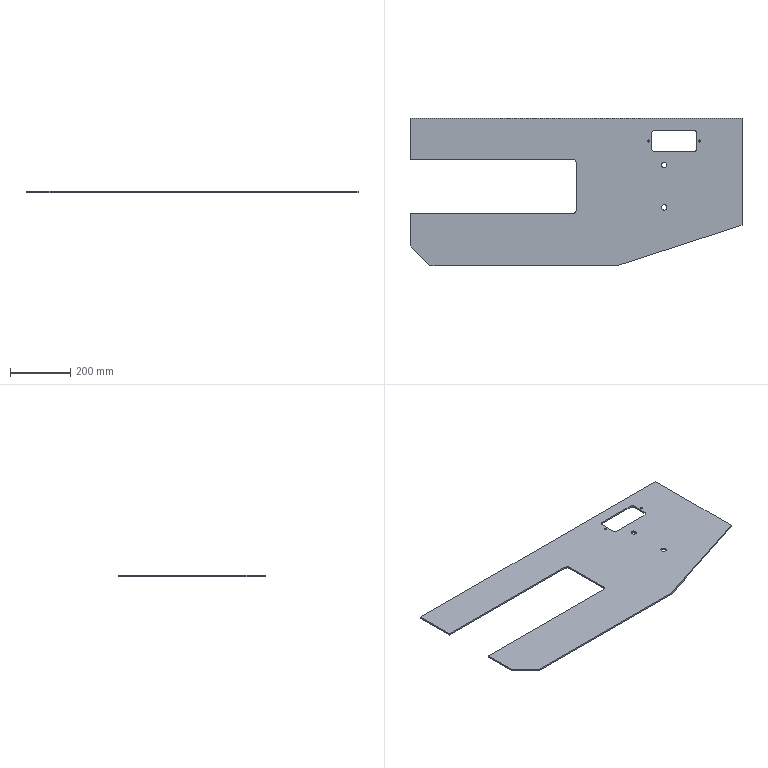Part | SolidWorks | features HoleWzd 2, FlatPattern 1, SMBaseFlange 1, SheetMetal 1 | 1 solid | 30 faces | box 1100 x 490 x 5 mm | volume 1994925 mm3 | plane 16 | cylinder 14 | commonest cylinder face diameters 20 x6 6.8 x4 17.5 x4
STEP:
#1=CARTESIAN_POINT('',(786.6,414.,-5.));
#2=VERTEX_POINT('',#1);
#3=CARTESIAN_POINT('',(793.4,414.,-5.));
#4=VERTEX_POINT('',#3);
#5=CARTESIAN_POINT('',(790.,414.,-5.));
#6=DIRECTION('',(0.,0.,1.));
#7=DIRECTION('',(1.,0.,0.));
#8=AXIS2_PLACEMENT_3D('',#5,#6,#7);
#9=CIRCLE('',#8,3.4);
#10=EDGE_CURVE('',#2,#4,#9,.T.);
#11=ORIENTED_EDGE('',*,*,#10,.F.);
#12=CARTESIAN_POINT('',(786.6,414.,0.));
#13=VERTEX_POINT('',#12);
#14=CARTESIAN_POINT('',(786.6,414.,0.));
#15=DIRECTION('',(0.,0.,1.));
#16=VECTOR('',#15,1000.);
#17=LINE('',#14,#16);
#18=EDGE_CURVE('',#2,#13,#17,.T.);
#19=ORIENTED_EDGE('',*,*,#18,.T.);
#20=CARTESIAN_POINT('',(793.4,414.,0.));
#21=VERTEX_POINT('',#20);
#22=CARTESIAN_POINT('',(790.,414.,0.));
#23=DIRECTION('',(0.,0.,1.));
#24=DIRECTION('',(1.,0.,0.));
#25=AXIS2_PLACEMENT_3D('',#22,#23,#24);
#26=CIRCLE('',#25,3.4);
#27=EDGE_CURVE('',#13,#21,#26,.T.);
#28=ORIENTED_EDGE('',*,*,#27,.T.);
#29=CARTESIAN_POINT('',(793.4,414.,0.));
#30=DIRECTION('',(0.,0.,1.));
#31=VECTOR('',#30,1000.);
#32=LINE('',#29,#31);
#33=EDGE_CURVE('',#4,#21,#32,.T.);
#34=ORIENTED_EDGE('',*,*,#33,.F.);
#35=EDGE_LOOP('',(#11,#19,#28,#34));
#36=FACE_OUTER_BOUND('',#35,.T.);
#37=CARTESIAN_POINT('',(790.,414.,0.));
#38=DIRECTION('',(0.,0.,1.));
#39=DIRECTION('',(1.,0.,0.));
#40=AXIS2_PLACEMENT_3D('',#37,#38,#39);
#41=CYLINDRICAL_SURFACE('',#40,3.4);
#42=ADVANCED_FACE('',(#36),#41,.F.);
#43=CARTESIAN_POINT('',(956.6,414.,-5.));
#44=VERTEX_POINT('',#43);
#45=CARTESIAN_POINT('',(963.4,414.,-5.));
#46=VERTEX_POINT('',#45);
#47=CARTESIAN_POINT('',(960.,414.,-5.));
#48=DIRECTION('',(0.,0.,1.));
#49=DIRECTION('',(1.,0.,0.));
#50=AXIS2_PLACEMENT_3D('',#47,#48,#49);
#51=CIRCLE('',#50,3.4);
#52=EDGE_CURVE('',#44,#46,#51,.T.);
#53=ORIENTED_EDGE('',*,*,#52,.F.);
#54=CARTESIAN_POINT('',(956.6,414.,0.));
#55=VERTEX_POINT('',#54);
#56=CARTESIAN_POINT('',(956.6,414.,0.));
#57=DIRECTION('',(0.,0.,1.));
#58=VECTOR('',#57,1000.);
#59=LINE('',#56,#58);
#60=EDGE_CURVE('',#44,#55,#59,.T.);
#61=ORIENTED_EDGE('',*,*,#60,.T.);
#62=CARTESIAN_POINT('',(963.4,414.,0.));
#63=VERTEX_POINT('',#62);
#64=CARTESIAN_POINT('',(960.,414.,0.));
#65=DIRECTION('',(0.,0.,1.));
#66=DIRECTION('',(1.,0.,0.));
#67=AXIS2_PLACEMENT_3D('',#64,#65,#66);
#68=CIRCLE('',#67,3.4);
#69=EDGE_CURVE('',#55,#63,#68,.T.);
#70=ORIENTED_EDGE('',*,*,#69,.T.);
#71=CARTESIAN_POINT('',(963.4,414.,0.));
#72=DIRECTION('',(0.,0.,1.));
#73=VECTOR('',#72,1000.);
#74=LINE('',#71,#73);
#75=EDGE_CURVE('',#46,#63,#74,.T.);
#76=ORIENTED_EDGE('',*,*,#75,.F.);
#77=EDGE_LOOP('',(#53,#61,#70,#76));
#78=FACE_OUTER_BOUND('',#77,.T.);
#79=CARTESIAN_POINT('',(960.,414.,0.));
#80=DIRECTION('',(0.,0.,1.));
#81=DIRECTION('',(1.,0.,0.));
#82=AXIS2_PLACEMENT_3D('',#79,#80,#81);
#83=CYLINDRICAL_SURFACE('',#82,3.4);
#84=ADVANCED_FACE('',(#78),#83,.F.);
#85=CARTESIAN_POINT('',(833.25,334.,-5.));
#86=VERTEX_POINT('',#85);
#87=CARTESIAN_POINT('',(850.75,334.,-5.));
#88=VERTEX_POINT('',#87);
#89=CARTESIAN_POINT('',(842.,334.,-5.));
#90=DIRECTION('',(0.,0.,1.));
#91=DIRECTION('',(1.,0.,0.));
#92=AXIS2_PLACEMENT_3D('',#89,#90,#91);
#93=CIRCLE('',#92,8.75);
#94=EDGE_CURVE('',#86,#88,#93,.T.);
#95=ORIENTED_EDGE('',*,*,#94,.F.);
#96=CARTESIAN_POINT('',(833.25,334.,0.));
#97=VERTEX_POINT('',#96);
#98=CARTESIAN_POINT('',(833.25,334.,0.));
#99=DIRECTION('',(0.,0.,1.));
#100=VECTOR('',#99,1000.);
#101=LINE('',#98,#100);
#102=EDGE_CURVE('',#86,#97,#101,.T.);
#103=ORIENTED_EDGE('',*,*,#102,.T.);
#104=CARTESIAN_POINT('',(850.75,334.,0.));
#105=VERTEX_POINT('',#104);
#106=CARTESIAN_POINT('',(842.,334.,0.));
#107=DIRECTION('',(0.,0.,1.));
#108=DIRECTION('',(1.,0.,0.));
#109=AXIS2_PLACEMENT_3D('',#106,#107,#108);
#110=CIRCLE('',#109,8.75);
#111=EDGE_CURVE('',#97,#105,#110,.T.);
#112=ORIENTED_EDGE('',*,*,#111,.T.);
#113=CARTESIAN_POINT('',(850.75,334.,0.));
#114=DIRECTION('',(0.,0.,1.));
#115=VECTOR('',#114,1000.);
#116=LINE('',#113,#115);
#117=EDGE_CURVE('',#88,#105,#116,.T.);
#118=ORIENTED_EDGE('',*,*,#117,.F.);
#119=EDGE_LOOP('',(#95,#103,#112,#118));
#120=FACE_OUTER_BOUND('',#119,.T.);
#121=CARTESIAN_POINT('',(842.,334.,0.));
#122=DIRECTION('',(0.,0.,1.));
#123=DIRECTION('',(1.,0.,0.));
#124=AXIS2_PLACEMENT_3D('',#121,#122,#123);
#125=CYLINDRICAL_SURFACE('',#124,8.75);
#126=ADVANCED_FACE('',(#120),#125,.F.);
#127=CARTESIAN_POINT('',(833.25,194.,-5.));
#128=VERTEX_POINT('',#127);
#129=CARTESIAN_POINT('',(850.75,194.,-5.));
#130=VERTEX_POINT('',#129);
#131=CARTESIAN_POINT('',(842.,194.,-5.));
#132=DIRECTION('',(0.,0.,1.));
#133=DIRECTION('',(1.,0.,0.));
#134=AXIS2_PLACEMENT_3D('',#131,#132,#133);
#135=CIRCLE('',#134,8.75);
#136=EDGE_CURVE('',#128,#130,#135,.T.);
#137=ORIENTED_EDGE('',*,*,#136,.F.);
#138=CARTESIAN_POINT('',(833.25,194.,0.));
#139=VERTEX_POINT('',#138);
#140=CARTESIAN_POINT('',(833.25,194.,0.));
#141=DIRECTION('',(0.,0.,1.));
#142=VECTOR('',#141,1000.);
#143=LINE('',#140,#142);
#144=EDGE_CURVE('',#128,#139,#143,.T.);
#145=ORIENTED_EDGE('',*,*,#144,.T.);
#146=CARTESIAN_POINT('',(850.75,194.,0.));
#147=VERTEX_POINT('',#146);
#148=CARTESIAN_POINT('',(842.,194.,0.));
#149=DIRECTION('',(0.,0.,1.));
#150=DIRECTION('',(1.,0.,0.));
#151=AXIS2_PLACEMENT_3D('',#148,#149,#150);
#152=CIRCLE('',#151,8.75);
#153=EDGE_CURVE('',#139,#147,#152,.T.);
#154=ORIENTED_EDGE('',*,*,#153,.T.);
#155=CARTESIAN_POINT('',(850.75,194.,0.));
#156=DIRECTION('',(0.,0.,1.));
#157=VECTOR('',#156,1000.);
#158=LINE('',#155,#157);
#159=EDGE_CURVE('',#130,#147,#158,.T.);
#160=ORIENTED_EDGE('',*,*,#159,.F.);
#161=EDGE_LOOP('',(#137,#145,#154,#160));
#162=FACE_OUTER_BOUND('',#161,.T.);
#163=CARTESIAN_POINT('',(842.,194.,0.));
#164=DIRECTION('',(0.,0.,1.));
#165=DIRECTION('',(1.,0.,0.));
#166=AXIS2_PLACEMENT_3D('',#163,#164,#165);
#167=CYLINDRICAL_SURFACE('',#166,8.75);
#168=ADVANCED_FACE('',(#162),#167,.F.);
#169=CARTESIAN_POINT('',(0.,490.,0.));
#170=VERTEX_POINT('',#169);
#171=CARTESIAN_POINT('',(0.,354.,0.));
#172=VERTEX_POINT('',#171);
#173=CARTESIAN_POINT('',(0.,354.,0.));
#174=DIRECTION('',(0.,-1.,0.));
#175=VECTOR('',#174,1000.);
#176=LINE('',#173,#175);
#177=EDGE_CURVE('',#170,#172,#176,.T.);
#178=ORIENTED_EDGE('',*,*,#177,.F.);
#179=CARTESIAN_POINT('',(0.,490.,-5.));
#180=VERTEX_POINT('',#179);
#181=CARTESIAN_POINT('',(0.,490.,-5.));
#182=DIRECTION('',(0.,0.,1.));
#183=VECTOR('',#182,1000.);
#184=LINE('',#181,#183);
#185=EDGE_CURVE('',#180,#170,#184,.T.);
#186=ORIENTED_EDGE('',*,*,#185,.F.);
#187=CARTESIAN_POINT('',(0.,354.,-5.));
#188=VERTEX_POINT('',#187);
#189=CARTESIAN_POINT('',(0.,354.,-5.));
#190=DIRECTION('',(0.,-1.,0.));
#191=VECTOR('',#190,1000.);
#192=LINE('',#189,#191);
#193=EDGE_CURVE('',#180,#188,#192,.T.);
#194=ORIENTED_EDGE('',*,*,#193,.T.);
#195=CARTESIAN_POINT('',(0.,354.,-5.));
#196=DIRECTION('',(0.,0.,1.));
#197=VECTOR('',#196,1000.);
#198=LINE('',#195,#197);
#199=EDGE_CURVE('',#188,#172,#198,.T.);
#200=ORIENTED_EDGE('',*,*,#199,.T.);
#201=EDGE_LOOP('',(#178,#186,#194,#200));
#202=FACE_OUTER_BOUND('',#201,.T.);
#203=CARTESIAN_POINT('',(0.,354.,-5.));
#204=DIRECTION('',(-1.,0.,0.));
#205=DIRECTION('',(0.,-1.,0.));
#206=AXIS2_PLACEMENT_3D('',#203,#204,#205);
#207=PLANE('',#206);
#208=ADVANCED_FACE('',(#202),#207,.T.);
#209=CARTESIAN_POINT('',(1100.,490.,0.));
#210=VERTEX_POINT('',#209);
#211=CARTESIAN_POINT('',(0.,490.,0.));
#212=DIRECTION('',(-1.,0.,0.));
#213=VECTOR('',#212,1000.);
#214=LINE('',#211,#213);
#215=EDGE_CURVE('',#210,#170,#214,.T.);
#216=ORIENTED_EDGE('',*,*,#215,.F.);
#217=CARTESIAN_POINT('',(1100.,490.,-5.));
#218=VERTEX_POINT('',#217);
#219=CARTESIAN_POINT('',(1100.,490.,-5.));
#220=DIRECTION('',(0.,0.,1.));
#221=VECTOR('',#220,1000.);
#222=LINE('',#219,#221);
#223=EDGE_CURVE('',#218,#210,#222,.T.);
#224=ORIENTED_EDGE('',*,*,#223,.F.);
#225=CARTESIAN_POINT('',(0.,490.,-5.));
#226=DIRECTION('',(-1.,0.,0.));
#227=VECTOR('',#226,1000.);
#228=LINE('',#225,#227);
#229=EDGE_CURVE('',#218,#180,#228,.T.);
#230=ORIENTED_EDGE('',*,*,#229,.T.);
#231=ORIENTED_EDGE('',*,*,#185,.T.);
#232=EDGE_LOOP('',(#216,#224,#230,#231));
#233=FACE_OUTER_BOUND('',#232,.T.);
#234=CARTESIAN_POINT('',(0.,490.,-5.));
#235=DIRECTION('',(0.,1.,0.));
#236=DIRECTION('',(0.,0.,1.));
#237=AXIS2_PLACEMENT_3D('',#234,#235,#236);
#238=PLANE('',#237);
#239=ADVANCED_FACE('',(#233),#238,.T.);
#240=CARTESIAN_POINT('',(1100.,134.647,0.));
#241=VERTEX_POINT('',#240);
#242=CARTESIAN_POINT('',(1100.,490.,0.));
#243=DIRECTION('',(0.,1.,0.));
#244=VECTOR('',#243,1000.);
#245=LINE('',#242,#244);
#246=EDGE_CURVE('',#241,#210,#245,.T.);
#247=ORIENTED_EDGE('',*,*,#246,.F.);
#248=CARTESIAN_POINT('',(1100.,134.647,-5.));
#249=VERTEX_POINT('',#248);
#250=CARTESIAN_POINT('',(1100.,134.647,-5.));
#251=DIRECTION('',(0.,0.,1.));
#252=VECTOR('',#251,1000.);
#253=LINE('',#250,#252);
#254=EDGE_CURVE('',#249,#241,#253,.T.);
#255=ORIENTED_EDGE('',*,*,#254,.F.);
#256=CARTESIAN_POINT('',(1100.,490.,-5.));
#257=DIRECTION('',(0.,1.,0.));
#258=VECTOR('',#257,1000.);
#259=LINE('',#256,#258);
#260=EDGE_CURVE('',#249,#218,#259,.T.);
#261=ORIENTED_EDGE('',*,*,#260,.T.);
#262=ORIENTED_EDGE('',*,*,#223,.T.);
#263=EDGE_LOOP('',(#247,#255,#261,#262));
#264=FACE_OUTER_BOUND('',#263,.T.);
#265=CARTESIAN_POINT('',(1100.,490.,-5.));
#266=DIRECTION('',(1.,0.,0.));
#267=DIRECTION('',(0.,0.,-1.));
#268=AXIS2_PLACEMENT_3D('',#265,#266,#267);
#269=PLANE('',#268);
#270=ADVANCED_FACE('',(#264),#269,.T.);
#271=CARTESIAN_POINT('',(685.6,0.,0.));
#272=VERTEX_POINT('',#271);
#273=CARTESIAN_POINT('',(1100.,134.647,0.));
#274=DIRECTION('',(0.9511,0.309,0.));
#275=VECTOR('',#274,1000.);
#276=LINE('',#273,#275);
#277=EDGE_CURVE('',#272,#241,#276,.T.);
#278=ORIENTED_EDGE('',*,*,#277,.F.);
#279=CARTESIAN_POINT('',(685.6,0.,-5.));
#280=VERTEX_POINT('',#279);
#281=CARTESIAN_POINT('',(685.6,0.,-5.));
#282=DIRECTION('',(0.,0.,1.));
#283=VECTOR('',#282,1000.);
#284=LINE('',#281,#283);
#285=EDGE_CURVE('',#280,#272,#284,.T.);
#286=ORIENTED_EDGE('',*,*,#285,.F.);
#287=CARTESIAN_POINT('',(1100.,134.647,-5.));
#288=DIRECTION('',(0.9511,0.309,0.));
#289=VECTOR('',#288,1000.);
#290=LINE('',#287,#289);
#291=EDGE_CURVE('',#280,#249,#290,.T.);
#292=ORIENTED_EDGE('',*,*,#291,.T.);
#293=ORIENTED_EDGE('',*,*,#254,.T.);
#294=EDGE_LOOP('',(#278,#286,#292,#293));
#295=FACE_OUTER_BOUND('',#294,.T.);
#296=CARTESIAN_POINT('',(1100.,134.647,-5.));
#297=DIRECTION('',(0.309,-0.9511,0.));
#298=DIRECTION('',(0.9511,0.309,0.));
#299=AXIS2_PLACEMENT_3D('',#296,#297,#298);
#300=PLANE('',#299);
#301=ADVANCED_FACE('',(#295),#300,.T.);
#302=CARTESIAN_POINT('',(66.2,0.,0.));
#303=VERTEX_POINT('',#302);
#304=CARTESIAN_POINT('',(685.6,0.,0.));
#305=DIRECTION('',(1.,0.,0.));
#306=VECTOR('',#305,1000.);
#307=LINE('',#304,#306);
#308=EDGE_CURVE('',#303,#272,#307,.T.);
#309=ORIENTED_EDGE('',*,*,#308,.F.);
#310=CARTESIAN_POINT('',(66.2,0.,-5.));
#311=VERTEX_POINT('',#310);
#312=CARTESIAN_POINT('',(66.2,0.,-5.));
#313=DIRECTION('',(0.,0.,1.));
#314=VECTOR('',#313,1000.);
#315=LINE('',#312,#314);
#316=EDGE_CURVE('',#311,#303,#315,.T.);
#317=ORIENTED_EDGE('',*,*,#316,.F.);
#318=CARTESIAN_POINT('',(685.6,0.,-5.));
#319=DIRECTION('',(1.,0.,0.));
#320=VECTOR('',#319,1000.);
#321=LINE('',#318,#320);
#322=EDGE_CURVE('',#311,#280,#321,.T.);
#323=ORIENTED_EDGE('',*,*,#322,.T.);
#324=ORIENTED_EDGE('',*,*,#285,.T.);
#325=EDGE_LOOP('',(#309,#317,#323,#324));
#326=FACE_OUTER_BOUND('',#325,.T.);
#327=CARTESIAN_POINT('',(685.6,0.,-5.));
#328=DIRECTION('',(0.,-1.,0.));
#329=DIRECTION('',(0.,0.,-1.));
#330=AXIS2_PLACEMENT_3D('',#327,#328,#329);
#331=PLANE('',#330);
#332=ADVANCED_FACE('',(#326),#331,.T.);
#333=CARTESIAN_POINT('',(0.,66.2,0.));
#334=VERTEX_POINT('',#333);
#335=CARTESIAN_POINT('',(66.2,0.,0.));
#336=DIRECTION('',(0.7071,-0.7071,0.));
#337=VECTOR('',#336,1000.);
#338=LINE('',#335,#337);
#339=EDGE_CURVE('',#334,#303,#338,.T.);
#340=ORIENTED_EDGE('',*,*,#339,.F.);
#341=CARTESIAN_POINT('',(0.,66.2,-5.));
#342=VERTEX_POINT('',#341);
#343=CARTESIAN_POINT('',(0.,66.2,-5.));
#344=DIRECTION('',(0.,0.,1.));
#345=VECTOR('',#344,1000.);
#346=LINE('',#343,#345);
#347=EDGE_CURVE('',#342,#334,#346,.T.);
#348=ORIENTED_EDGE('',*,*,#347,.F.);
#349=CARTESIAN_POINT('',(66.2,0.,-5.));
#350=DIRECTION('',(0.7071,-0.7071,0.));
#351=VECTOR('',#350,1000.);
#352=LINE('',#349,#351);
#353=EDGE_CURVE('',#342,#311,#352,.T.);
#354=ORIENTED_EDGE('',*,*,#353,.T.);
#355=ORIENTED_EDGE('',*,*,#316,.T.);
#356=EDGE_LOOP('',(#340,#348,#354,#355));
#357=FACE_OUTER_BOUND('',#356,.T.);
#358=CARTESIAN_POINT('',(66.2,0.,-5.));
#359=DIRECTION('',(-0.7071,-0.7071,0.));
#360=DIRECTION('',(0.7071,-0.7071,0.));
#361=AXIS2_PLACEMENT_3D('',#358,#359,#360);
#362=PLANE('',#361);
#363=ADVANCED_FACE('',(#357),#362,.T.);
#364=CARTESIAN_POINT('',(0.,174.,0.));
#365=VERTEX_POINT('',#364);
#366=CARTESIAN_POINT('',(0.,66.2,0.));
#367=DIRECTION('',(0.,-1.,0.));
#368=VECTOR('',#367,1000.);
#369=LINE('',#366,#368);
#370=EDGE_CURVE('',#365,#334,#369,.T.);
#371=ORIENTED_EDGE('',*,*,#370,.F.);
#372=CARTESIAN_POINT('',(0.,174.,-5.));
#373=VERTEX_POINT('',#372);
#374=CARTESIAN_POINT('',(0.,174.,-5.));
#375=DIRECTION('',(0.,0.,1.));
#376=VECTOR('',#375,1000.);
#377=LINE('',#374,#376);
#378=EDGE_CURVE('',#373,#365,#377,.T.);
#379=ORIENTED_EDGE('',*,*,#378,.F.);
#380=CARTESIAN_POINT('',(0.,66.2,-5.));
#381=DIRECTION('',(0.,-1.,0.));
#382=VECTOR('',#381,1000.);
#383=LINE('',#380,#382);
#384=EDGE_CURVE('',#373,#342,#383,.T.);
#385=ORIENTED_EDGE('',*,*,#384,.T.);
#386=ORIENTED_EDGE('',*,*,#347,.T.);
#387=EDGE_LOOP('',(#371,#379,#385,#386));
#388=FACE_OUTER_BOUND('',#387,.T.);
#389=CARTESIAN_POINT('',(0.,66.2,-5.));
#390=DIRECTION('',(-1.,0.,0.));
#391=DIRECTION('',(0.,-1.,0.));
#392=AXIS2_PLACEMENT_3D('',#389,#390,#391);
#393=PLANE('',#392);
#394=ADVANCED_FACE('',(#388),#393,.T.);
#395=CARTESIAN_POINT('',(540.,174.,0.));
#396=VERTEX_POINT('',#395);
#397=CARTESIAN_POINT('',(540.,174.,0.));
#398=DIRECTION('',(-1.,0.,0.));
#399=VECTOR('',#398,1000.);
#400=LINE('',#397,#399);
#401=EDGE_CURVE('',#396,#365,#400,.T.);
#402=ORIENTED_EDGE('',*,*,#401,.F.);
#403=CARTESIAN_POINT('',(540.,174.,-5.));
#404=VERTEX_POINT('',#403);
#405=CARTESIAN_POINT('',(540.,174.,-5.));
#406=DIRECTION('',(0.,0.,1.));
#407=VECTOR('',#406,1000.);
#408=LINE('',#405,#407);
#409=EDGE_CURVE('',#404,#396,#408,.T.);
#410=ORIENTED_EDGE('',*,*,#409,.F.);
#411=CARTESIAN_POINT('',(540.,174.,-5.));
#412=DIRECTION('',(-1.,0.,0.));
#413=VECTOR('',#412,1000.);
#414=LINE('',#411,#413);
#415=EDGE_CURVE('',#404,#373,#414,.T.);
#416=ORIENTED_EDGE('',*,*,#415,.T.);
#417=ORIENTED_EDGE('',*,*,#378,.T.);
#418=EDGE_LOOP('',(#402,#410,#416,#417));
#419=FACE_OUTER_BOUND('',#418,.T.);
#420=CARTESIAN_POINT('',(540.,174.,-5.));
#421=DIRECTION('',(0.,1.,0.));
#422=DIRECTION('',(-1.,0.,0.));
#423=AXIS2_PLACEMENT_3D('',#420,#421,#422);
#424=PLANE('',#423);
#425=ADVANCED_FACE('',(#419),#424,.T.);
#426=CARTESIAN_POINT('',(550.,184.,0.));
#427=VERTEX_POINT('',#426);
#428=CARTESIAN_POINT('',(540.,184.,0.));
#429=DIRECTION('',(0.,0.,-1.));
#430=DIRECTION('',(1.,0.,0.));
#431=AXIS2_PLACEMENT_3D('',#428,#429,#430);
#432=CIRCLE('',#431,10.);
#433=EDGE_CURVE('',#427,#396,#432,.T.);
#434=ORIENTED_EDGE('',*,*,#433,.F.);
#435=CARTESIAN_POINT('',(550.,184.,-5.));
#436=VERTEX_POINT('',#435);
#437=CARTESIAN_POINT('',(550.,184.,-5.));
#438=DIRECTION('',(0.,0.,1.));
#439=VECTOR('',#438,1000.);
#440=LINE('',#437,#439);
#441=EDGE_CURVE('',#436,#427,#440,.T.);
#442=ORIENTED_EDGE('',*,*,#441,.F.);
#443=CARTESIAN_POINT('',(540.,184.,-5.));
#444=DIRECTION('',(0.,0.,-1.));
#445=DIRECTION('',(1.,0.,0.));
#446=AXIS2_PLACEMENT_3D('',#443,#444,#445);
#447=CIRCLE('',#446,10.);
#448=EDGE_CURVE('',#436,#404,#447,.T.);
#449=ORIENTED_EDGE('',*,*,#448,.T.);
#450=ORIENTED_EDGE('',*,*,#409,.T.);
#451=EDGE_LOOP('',(#434,#442,#449,#450));
#452=FACE_OUTER_BOUND('',#451,.T.);
#453=CARTESIAN_POINT('',(540.,184.,-5.));
#454=DIRECTION('',(0.,0.,1.));
#455=DIRECTION('',(1.,0.,0.));
#456=AXIS2_PLACEMENT_3D('',#453,#454,#455);
#457=CYLINDRICAL_SURFACE('',#456,10.);
#458=ADVANCED_FACE('',(#452),#457,.F.);
#459=CARTESIAN_POINT('',(550.,344.,0.));
#460=VERTEX_POINT('',#459);
#461=CARTESIAN_POINT('',(550.,344.,0.));
#462=DIRECTION('',(0.,-1.,0.));
#463=VECTOR('',#462,1000.);
#464=LINE('',#461,#463);
#465=EDGE_CURVE('',#460,#427,#464,.T.);
#466=ORIENTED_EDGE('',*,*,#465,.F.);
#467=CARTESIAN_POINT('',(550.,344.,-5.));
#468=VERTEX_POINT('',#467);
#469=CARTESIAN_POINT('',(550.,344.,-5.));
#470=DIRECTION('',(0.,0.,1.));
#471=VECTOR('',#470,1000.);
#472=LINE('',#469,#471);
#473=EDGE_CURVE('',#468,#460,#472,.T.);
#474=ORIENTED_EDGE('',*,*,#473,.F.);
#475=CARTESIAN_POINT('',(550.,344.,-5.));
#476=DIRECTION('',(0.,-1.,0.));
#477=VECTOR('',#476,1000.);
#478=LINE('',#475,#477);
#479=EDGE_CURVE('',#468,#436,#478,.T.);
#480=ORIENTED_EDGE('',*,*,#479,.T.);
#481=ORIENTED_EDGE('',*,*,#441,.T.);
#482=EDGE_LOOP('',(#466,#474,#480,#481));
#483=FACE_OUTER_BOUND('',#482,.T.);
#484=CARTESIAN_POINT('',(550.,344.,-5.));
#485=DIRECTION('',(-1.,0.,0.));
#486=DIRECTION('',(0.,0.,1.));
#487=AXIS2_PLACEMENT_3D('',#484,#485,#486);
#488=PLANE('',#487);
#489=ADVANCED_FACE('',(#483),#488,.T.);
#490=CARTESIAN_POINT('',(540.,354.,0.));
#491=VERTEX_POINT('',#490);
#492=CARTESIAN_POINT('',(540.,344.,0.));
#493=DIRECTION('',(0.,0.,-1.));
#494=DIRECTION('',(1.,0.,0.));
#495=AXIS2_PLACEMENT_3D('',#492,#493,#494);
#496=CIRCLE('',#495,10.);
#497=EDGE_CURVE('',#491,#460,#496,.T.);
#498=ORIENTED_EDGE('',*,*,#497,.F.);
#499=CARTESIAN_POINT('',(540.,354.,-5.));
#500=VERTEX_POINT('',#499);
#501=CARTESIAN_POINT('',(540.,354.,-5.));
#502=DIRECTION('',(0.,0.,1.));
#503=VECTOR('',#502,1000.);
#504=LINE('',#501,#503);
#505=EDGE_CURVE('',#500,#491,#504,.T.);
#506=ORIENTED_EDGE('',*,*,#505,.F.);
#507=CARTESIAN_POINT('',(540.,344.,-5.));
#508=DIRECTION('',(0.,0.,-1.));
#509=DIRECTION('',(1.,0.,0.));
#510=AXIS2_PLACEMENT_3D('',#507,#508,#509);
#511=CIRCLE('',#510,10.);
#512=EDGE_CURVE('',#500,#468,#511,.T.);
#513=ORIENTED_EDGE('',*,*,#512,.T.);
#514=ORIENTED_EDGE('',*,*,#473,.T.);
#515=EDGE_LOOP('',(#498,#506,#513,#514));
#516=FACE_OUTER_BOUND('',#515,.T.);
#517=CARTESIAN_POINT('',(540.,344.,-5.));
#518=DIRECTION('',(0.,0.,1.));
#519=DIRECTION('',(1.,0.,0.));
#520=AXIS2_PLACEMENT_3D('',#517,#518,#519);
#521=CYLINDRICAL_SURFACE('',#520,10.);
#522=ADVANCED_FACE('',(#516),#521,.F.);
#523=CARTESIAN_POINT('',(0.,354.,0.));
#524=DIRECTION('',(1.,0.,0.));
#525=VECTOR('',#524,1000.);
#526=LINE('',#523,#525);
#527=EDGE_CURVE('',#172,#491,#526,.T.);
#528=ORIENTED_EDGE('',*,*,#527,.F.);
#529=ORIENTED_EDGE('',*,*,#199,.F.);
#530=CARTESIAN_POINT('',(0.,354.,-5.));
#531=DIRECTION('',(1.,0.,0.));
#532=VECTOR('',#531,1000.);
#533=LINE('',#530,#532);
#534=EDGE_CURVE('',#188,#500,#533,.T.);
#535=ORIENTED_EDGE('',*,*,#534,.T.);
#536=ORIENTED_EDGE('',*,*,#505,.T.);
#537=EDGE_LOOP('',(#528,#529,#535,#536));
#538=FACE_OUTER_BOUND('',#537,.T.);
#539=CARTESIAN_POINT('',(0.,354.,-5.));
#540=DIRECTION('',(0.,-1.,0.));
#541=DIRECTION('',(0.,0.,-1.));
#542=AXIS2_PLACEMENT_3D('',#539,#540,#541);
#543=PLANE('',#542);
#544=ADVANCED_FACE('',(#538),#543,.T.);
#545=CARTESIAN_POINT('',(790.,414.,-5.));
#546=DIRECTION('',(0.,0.,1.));
#547=DIRECTION('',(1.,0.,0.));
#548=AXIS2_PLACEMENT_3D('',#545,#546,#547);
#549=CIRCLE('',#548,3.4);
#550=EDGE_CURVE('',#4,#2,#549,.T.);
#551=ORIENTED_EDGE('',*,*,#550,.T.);
#552=ORIENTED_EDGE('',*,*,#10,.T.);
#553=EDGE_LOOP('',(#551,#552));
#554=FACE_BOUND('',#553,.T.);
#555=CARTESIAN_POINT('',(960.,414.,-5.));
#556=DIRECTION('',(0.,0.,1.));
#557=DIRECTION('',(1.,0.,0.));
#558=AXIS2_PLACEMENT_3D('',#555,#556,#557);
#559=CIRCLE('',#558,3.4);
#560=EDGE_CURVE('',#46,#44,#559,.T.);
#561=ORIENTED_EDGE('',*,*,#560,.T.);
#562=ORIENTED_EDGE('',*,*,#52,.T.);
#563=EDGE_LOOP('',(#561,#562));
#564=FACE_BOUND('',#563,.T.);
#565=CARTESIAN_POINT('',(842.,334.,-5.));
#566=DIRECTION('',(0.,0.,1.));
#567=DIRECTION('',(1.,0.,0.));
#568=AXIS2_PLACEMENT_3D('',#565,#566,#567);
#569=CIRCLE('',#568,8.75);
#570=EDGE_CURVE('',#88,#86,#569,.T.);
#571=ORIENTED_EDGE('',*,*,#570,.T.);
#572=ORIENTED_EDGE('',*,*,#94,.T.);
#573=EDGE_LOOP('',(#571,#572));
#574=FACE_BOUND('',#573,.T.);
#575=CARTESIAN_POINT('',(842.,194.,-5.));
#576=DIRECTION('',(0.,0.,1.));
#577=DIRECTION('',(1.,0.,0.));
#578=AXIS2_PLACEMENT_3D('',#575,#576,#577);
#579=CIRCLE('',#578,8.75);
#580=EDGE_CURVE('',#130,#128,#579,.T.);
#581=ORIENTED_EDGE('',*,*,#580,.T.);
#582=ORIENTED_EDGE('',*,*,#136,.T.);
#583=EDGE_LOOP('',(#581,#582));
#584=FACE_BOUND('',#583,.T.);
#585=CARTESIAN_POINT('',(810.,379.,-5.));
#586=VERTEX_POINT('',#585);
#587=CARTESIAN_POINT('',(940.,379.,-5.));
#588=VERTEX_POINT('',#587);
#589=CARTESIAN_POINT('',(810.,379.,-5.));
#590=DIRECTION('',(1.,0.,0.));
#591=VECTOR('',#590,1000.);
#592=LINE('',#589,#591);
#593=EDGE_CURVE('',#586,#588,#592,.T.);
#594=ORIENTED_EDGE('',*,*,#593,.T.);
#595=CARTESIAN_POINT('',(950.,389.,-5.));
#596=VERTEX_POINT('',#595);
#597=CARTESIAN_POINT('',(940.,389.,-5.));
#598=DIRECTION('',(0.,0.,1.));
#599=DIRECTION('',(1.,0.,0.));
#600=AXIS2_PLACEMENT_3D('',#597,#598,#599);
#601=CIRCLE('',#600,10.);
#602=EDGE_CURVE('',#588,#596,#601,.T.);
#603=ORIENTED_EDGE('',*,*,#602,.T.);
#604=CARTESIAN_POINT('',(950.,439.,-5.));
#605=VERTEX_POINT('',#604);
#606=CARTESIAN_POINT('',(950.,439.,-5.));
#607=DIRECTION('',(0.,1.,0.));
#608=VECTOR('',#607,1000.);
#609=LINE('',#606,#608);
#610=EDGE_CURVE('',#596,#605,#609,.T.);
#611=ORIENTED_EDGE('',*,*,#610,.T.);
#612=CARTESIAN_POINT('',(940.,449.,-5.));
#613=VERTEX_POINT('',#612);
#614=CARTESIAN_POINT('',(940.,439.,-5.));
#615=DIRECTION('',(0.,0.,1.));
#616=DIRECTION('',(1.,0.,0.));
#617=AXIS2_PLACEMENT_3D('',#614,#615,#616);
#618=CIRCLE('',#617,10.);
#619=EDGE_CURVE('',#605,#613,#618,.T.);
#620=ORIENTED_EDGE('',*,*,#619,.T.);
#621=CARTESIAN_POINT('',(810.,449.,-5.));
#622=VERTEX_POINT('',#621);
#623=CARTESIAN_POINT('',(810.,449.,-5.));
#624=DIRECTION('',(-1.,0.,0.));
#625=VECTOR('',#624,1000.);
#626=LINE('',#623,#625);
#627=EDGE_CURVE('',#613,#622,#626,.T.);
#628=ORIENTED_EDGE('',*,*,#627,.T.);
#629=CARTESIAN_POINT('',(800.,439.,-5.));
#630=VERTEX_POINT('',#629);
#631=CARTESIAN_POINT('',(810.,439.,-5.));
#632=DIRECTION('',(0.,0.,1.));
#633=DIRECTION('',(1.,0.,0.));
#634=AXIS2_PLACEMENT_3D('',#631,#632,#633);
#635=CIRCLE('',#634,10.);
#636=EDGE_CURVE('',#622,#630,#635,.T.);
#637=ORIENTED_EDGE('',*,*,#636,.T.);
#638=CARTESIAN_POINT('',(800.,389.,-5.));
#639=VERTEX_POINT('',#638);
#640=CARTESIAN_POINT('',(800.,439.,-5.));
#641=DIRECTION('',(0.,-1.,0.));
#642=VECTOR('',#641,1000.);
#643=LINE('',#640,#642);
#644=EDGE_CURVE('',#630,#639,#643,.T.);
#645=ORIENTED_EDGE('',*,*,#644,.T.);
#646=CARTESIAN_POINT('',(810.,389.,-5.));
#647=DIRECTION('',(0.,0.,1.));
#648=DIRECTION('',(-1.,0.,0.));
#649=AXIS2_PLACEMENT_3D('',#646,#647,#648);
#650=CIRCLE('',#649,10.);
#651=EDGE_CURVE('',#639,#586,#650,.T.);
#652=ORIENTED_EDGE('',*,*,#651,.T.);
#653=EDGE_LOOP('',(#594,#603,#611,#620,#628,#637,#645,#652));
#654=FACE_BOUND('',#653,.T.);
#655=ORIENTED_EDGE('',*,*,#193,.F.);
#656=ORIENTED_EDGE('',*,*,#229,.F.);
#657=ORIENTED_EDGE('',*,*,#260,.F.);
#658=ORIENTED_EDGE('',*,*,#291,.F.);
#659=ORIENTED_EDGE('',*,*,#322,.F.);
#660=ORIENTED_EDGE('',*,*,#353,.F.);
#661=ORIENTED_EDGE('',*,*,#384,.F.);
#662=ORIENTED_EDGE('',*,*,#415,.F.);
#663=ORIENTED_EDGE('',*,*,#448,.F.);
#664=ORIENTED_EDGE('',*,*,#479,.F.);
#665=ORIENTED_EDGE('',*,*,#512,.F.);
#666=ORIENTED_EDGE('',*,*,#534,.F.);
#667=EDGE_LOOP('',(#655,#656,#657,#658,#659,#660,#661,#662,#663,#664,#665,#666));
#668=FACE_OUTER_BOUND('',#667,.T.);
#669=CARTESIAN_POINT('',(540.,184.,-5.));
#670=DIRECTION('',(0.,0.,1.));
#671=DIRECTION('',(1.,0.,0.));
#672=AXIS2_PLACEMENT_3D('',#669,#670,#671);
#673=PLANE('',#672);
#674=ADVANCED_FACE('',(#554,#564,#574,#584,#654,#668),#673,.F.);
#675=CARTESIAN_POINT('',(790.,414.,0.));
#676=DIRECTION('',(0.,0.,1.));
#677=DIRECTION('',(1.,0.,0.));
#678=AXIS2_PLACEMENT_3D('',#675,#676,#677);
#679=CIRCLE('',#678,3.4);
#680=EDGE_CURVE('',#21,#13,#679,.T.);
#681=ORIENTED_EDGE('',*,*,#680,.F.);
#682=ORIENTED_EDGE('',*,*,#27,.F.);
#683=EDGE_LOOP('',(#681,#682));
#684=FACE_BOUND('',#683,.T.);
#685=CARTESIAN_POINT('',(960.,414.,0.));
#686=DIRECTION('',(0.,0.,1.));
#687=DIRECTION('',(1.,0.,0.));
#688=AXIS2_PLACEMENT_3D('',#685,#686,#687);
#689=CIRCLE('',#688,3.4);
#690=EDGE_CURVE('',#63,#55,#689,.T.);
#691=ORIENTED_EDGE('',*,*,#690,.F.);
#692=ORIENTED_EDGE('',*,*,#69,.F.);
#693=EDGE_LOOP('',(#691,#692));
#694=FACE_BOUND('',#693,.T.);
#695=CARTESIAN_POINT('',(842.,334.,0.));
#696=DIRECTION('',(0.,0.,1.));
#697=DIRECTION('',(1.,0.,0.));
#698=AXIS2_PLACEMENT_3D('',#695,#696,#697);
#699=CIRCLE('',#698,8.75);
#700=EDGE_CURVE('',#105,#97,#699,.T.);
#701=ORIENTED_EDGE('',*,*,#700,.F.);
#702=ORIENTED_EDGE('',*,*,#111,.F.);
#703=EDGE_LOOP('',(#701,#702));
#704=FACE_BOUND('',#703,.T.);
#705=CARTESIAN_POINT('',(842.,194.,0.));
#706=DIRECTION('',(0.,0.,1.));
#707=DIRECTION('',(1.,0.,0.));
#708=AXIS2_PLACEMENT_3D('',#705,#706,#707);
#709=CIRCLE('',#708,8.75);
#710=EDGE_CURVE('',#147,#139,#709,.T.);
#711=ORIENTED_EDGE('',*,*,#710,.F.);
#712=ORIENTED_EDGE('',*,*,#153,.F.);
#713=EDGE_LOOP('',(#711,#712));
#714=FACE_BOUND('',#713,.T.);
#715=CARTESIAN_POINT('',(940.,379.,0.));
#716=VERTEX_POINT('',#715);
#717=CARTESIAN_POINT('',(950.,389.,0.));
#718=VERTEX_POINT('',#717);
#719=CARTESIAN_POINT('',(940.,389.,0.));
#720=DIRECTION('',(0.,0.,1.));
#721=DIRECTION('',(1.,0.,0.));
#722=AXIS2_PLACEMENT_3D('',#719,#720,#721);
#723=CIRCLE('',#722,10.);
#724=EDGE_CURVE('',#716,#718,#723,.T.);
#725=ORIENTED_EDGE('',*,*,#724,.F.);
#726=CARTESIAN_POINT('',(810.,379.,0.));
#727=VERTEX_POINT('',#726);
#728=CARTESIAN_POINT('',(810.,379.,0.));
#729=DIRECTION('',(1.,0.,0.));
#730=VECTOR('',#729,1000.);
#731=LINE('',#728,#730);
#732=EDGE_CURVE('',#727,#716,#731,.T.);
#733=ORIENTED_EDGE('',*,*,#732,.F.);
#734=CARTESIAN_POINT('',(800.,389.,0.));
#735=VERTEX_POINT('',#734);
#736=CARTESIAN_POINT('',(810.,389.,0.));
#737=DIRECTION('',(0.,0.,1.));
#738=DIRECTION('',(-1.,0.,0.));
#739=AXIS2_PLACEMENT_3D('',#736,#737,#738);
#740=CIRCLE('',#739,10.);
#741=EDGE_CURVE('',#735,#727,#740,.T.);
#742=ORIENTED_EDGE('',*,*,#741,.F.);
#743=CARTESIAN_POINT('',(800.,439.,0.));
#744=VERTEX_POINT('',#743);
#745=CARTESIAN_POINT('',(800.,439.,0.));
#746=DIRECTION('',(0.,-1.,0.));
#747=VECTOR('',#746,1000.);
#748=LINE('',#745,#747);
#749=EDGE_CURVE('',#744,#735,#748,.T.);
#750=ORIENTED_EDGE('',*,*,#749,.F.);
#751=CARTESIAN_POINT('',(810.,449.,0.));
#752=VERTEX_POINT('',#751);
#753=CARTESIAN_POINT('',(810.,439.,0.));
#754=DIRECTION('',(0.,0.,1.));
#755=DIRECTION('',(1.,0.,0.));
#756=AXIS2_PLACEMENT_3D('',#753,#754,#755);
#757=CIRCLE('',#756,10.);
#758=EDGE_CURVE('',#752,#744,#757,.T.);
#759=ORIENTED_EDGE('',*,*,#758,.F.);
#760=CARTESIAN_POINT('',(940.,449.,0.));
#761=VERTEX_POINT('',#760);
#762=CARTESIAN_POINT('',(810.,449.,0.));
#763=DIRECTION('',(-1.,0.,0.));
#764=VECTOR('',#763,1000.);
#765=LINE('',#762,#764);
#766=EDGE_CURVE('',#761,#752,#765,.T.);
#767=ORIENTED_EDGE('',*,*,#766,.F.);
#768=CARTESIAN_POINT('',(950.,439.,0.));
#769=VERTEX_POINT('',#768);
#770=CARTESIAN_POINT('',(940.,439.,0.));
#771=DIRECTION('',(0.,0.,1.));
#772=DIRECTION('',(1.,0.,0.));
#773=AXIS2_PLACEMENT_3D('',#770,#771,#772);
#774=CIRCLE('',#773,10.);
#775=EDGE_CURVE('',#769,#761,#774,.T.);
#776=ORIENTED_EDGE('',*,*,#775,.F.);
#777=CARTESIAN_POINT('',(950.,439.,0.));
#778=DIRECTION('',(0.,1.,0.));
#779=VECTOR('',#778,1000.);
#780=LINE('',#777,#779);
#781=EDGE_CURVE('',#718,#769,#780,.T.);
#782=ORIENTED_EDGE('',*,*,#781,.F.);
#783=EDGE_LOOP('',(#725,#733,#742,#750,#759,#767,#776,#782));
#784=FACE_BOUND('',#783,.T.);
#785=ORIENTED_EDGE('',*,*,#177,.T.);
#786=ORIENTED_EDGE('',*,*,#527,.T.);
#787=ORIENTED_EDGE('',*,*,#497,.T.);
#788=ORIENTED_EDGE('',*,*,#465,.T.);
#789=ORIENTED_EDGE('',*,*,#433,.T.);
#790=ORIENTED_EDGE('',*,*,#401,.T.);
#791=ORIENTED_EDGE('',*,*,#370,.T.);
#792=ORIENTED_EDGE('',*,*,#339,.T.);
#793=ORIENTED_EDGE('',*,*,#308,.T.);
#794=ORIENTED_EDGE('',*,*,#277,.T.);
#795=ORIENTED_EDGE('',*,*,#246,.T.);
#796=ORIENTED_EDGE('',*,*,#215,.T.);
#797=EDGE_LOOP('',(#785,#786,#787,#788,#789,#790,#791,#792,#793,#794,#795,#796));
#798=FACE_OUTER_BOUND('',#797,.T.);
#799=CARTESIAN_POINT('',(540.,184.,0.));
#800=DIRECTION('',(0.,0.,1.));
#801=DIRECTION('',(1.,0.,0.));
#802=AXIS2_PLACEMENT_3D('',#799,#800,#801);
#803=PLANE('',#802);
#804=ADVANCED_FACE('',(#684,#694,#704,#714,#784,#798),#803,.T.);
#805=ORIENTED_EDGE('',*,*,#724,.T.);
#806=CARTESIAN_POINT('',(950.,389.,-5.));
#807=DIRECTION('',(0.,0.,1.));
#808=VECTOR('',#807,1000.);
#809=LINE('',#806,#808);
#810=EDGE_CURVE('',#596,#718,#809,.T.);
#811=ORIENTED_EDGE('',*,*,#810,.F.);
#812=ORIENTED_EDGE('',*,*,#602,.F.);
#813=CARTESIAN_POINT('',(940.,379.,-5.));
#814=DIRECTION('',(0.,0.,1.));
#815=VECTOR('',#814,1000.);
#816=LINE('',#813,#815);
#817=EDGE_CURVE('',#588,#716,#816,.T.);
#818=ORIENTED_EDGE('',*,*,#817,.T.);
#819=EDGE_LOOP('',(#805,#811,#812,#818));
#820=FACE_OUTER_BOUND('',#819,.T.);
#821=CARTESIAN_POINT('',(940.,389.,-5.));
#822=DIRECTION('',(0.,0.,1.));
#823=DIRECTION('',(1.,0.,0.));
#824=AXIS2_PLACEMENT_3D('',#821,#822,#823);
#825=CYLINDRICAL_SURFACE('',#824,10.);
#826=ADVANCED_FACE('',(#820),#825,.F.);
#827=ORIENTED_EDGE('',*,*,#732,.T.);
#828=ORIENTED_EDGE('',*,*,#817,.F.);
#829=ORIENTED_EDGE('',*,*,#593,.F.);
#830=CARTESIAN_POINT('',(810.,379.,-5.));
#831=DIRECTION('',(0.,0.,1.));
#832=VECTOR('',#831,1000.);
#833=LINE('',#830,#832);
#834=EDGE_CURVE('',#586,#727,#833,.T.);
#835=ORIENTED_EDGE('',*,*,#834,.T.);
#836=EDGE_LOOP('',(#827,#828,#829,#835));
#837=FACE_OUTER_BOUND('',#836,.T.);
#838=CARTESIAN_POINT('',(810.,379.,-5.));
#839=DIRECTION('',(0.,-1.,0.));
#840=DIRECTION('',(1.,0.,0.));
#841=AXIS2_PLACEMENT_3D('',#838,#839,#840);
#842=PLANE('',#841);
#843=ADVANCED_FACE('',(#837),#842,.F.);
#844=ORIENTED_EDGE('',*,*,#741,.T.);
#845=ORIENTED_EDGE('',*,*,#834,.F.);
#846=ORIENTED_EDGE('',*,*,#651,.F.);
#847=CARTESIAN_POINT('',(800.,389.,-5.));
#848=DIRECTION('',(0.,0.,1.));
#849=VECTOR('',#848,1000.);
#850=LINE('',#847,#849);
#851=EDGE_CURVE('',#639,#735,#850,.T.);
#852=ORIENTED_EDGE('',*,*,#851,.T.);
#853=EDGE_LOOP('',(#844,#845,#846,#852));
#854=FACE_OUTER_BOUND('',#853,.T.);
#855=CARTESIAN_POINT('',(810.,389.,-5.));
#856=DIRECTION('',(0.,0.,1.));
#857=DIRECTION('',(1.,0.,0.));
#858=AXIS2_PLACEMENT_3D('',#855,#856,#857);
#859=CYLINDRICAL_SURFACE('',#858,10.);
#860=ADVANCED_FACE('',(#854),#859,.F.);
#861=ORIENTED_EDGE('',*,*,#749,.T.);
#862=ORIENTED_EDGE('',*,*,#851,.F.);
#863=ORIENTED_EDGE('',*,*,#644,.F.);
#864=CARTESIAN_POINT('',(800.,439.,-5.));
#865=DIRECTION('',(0.,0.,1.));
#866=VECTOR('',#865,1000.);
#867=LINE('',#864,#866);
#868=EDGE_CURVE('',#630,#744,#867,.T.);
#869=ORIENTED_EDGE('',*,*,#868,.T.);
#870=EDGE_LOOP('',(#861,#862,#863,#869));
#871=FACE_OUTER_BOUND('',#870,.T.);
#872=CARTESIAN_POINT('',(800.,439.,-5.));
#873=DIRECTION('',(-1.,0.,0.));
#874=DIRECTION('',(0.,0.,1.));
#875=AXIS2_PLACEMENT_3D('',#872,#873,#874);
#876=PLANE('',#875);
#877=ADVANCED_FACE('',(#871),#876,.F.);
#878=ORIENTED_EDGE('',*,*,#758,.T.);
#879=ORIENTED_EDGE('',*,*,#868,.F.);
#880=ORIENTED_EDGE('',*,*,#636,.F.);
#881=CARTESIAN_POINT('',(810.,449.,-5.));
#882=DIRECTION('',(0.,0.,1.));
#883=VECTOR('',#882,1000.);
#884=LINE('',#881,#883);
#885=EDGE_CURVE('',#622,#752,#884,.T.);
#886=ORIENTED_EDGE('',*,*,#885,.T.);
#887=EDGE_LOOP('',(#878,#879,#880,#886));
#888=FACE_OUTER_BOUND('',#887,.T.);
#889=CARTESIAN_POINT('',(810.,439.,-5.));
#890=DIRECTION('',(0.,0.,1.));
#891=DIRECTION('',(1.,0.,0.));
#892=AXIS2_PLACEMENT_3D('',#889,#890,#891);
#893=CYLINDRICAL_SURFACE('',#892,10.);
#894=ADVANCED_FACE('',(#888),#893,.F.);
#895=ORIENTED_EDGE('',*,*,#766,.T.);
#896=ORIENTED_EDGE('',*,*,#885,.F.);
#897=ORIENTED_EDGE('',*,*,#627,.F.);
#898=CARTESIAN_POINT('',(940.,449.,-5.));
#899=DIRECTION('',(0.,0.,1.));
#900=VECTOR('',#899,1000.);
#901=LINE('',#898,#900);
#902=EDGE_CURVE('',#613,#761,#901,.T.);
#903=ORIENTED_EDGE('',*,*,#902,.T.);
#904=EDGE_LOOP('',(#895,#896,#897,#903));
#905=FACE_OUTER_BOUND('',#904,.T.);
#906=CARTESIAN_POINT('',(810.,449.,-5.));
#907=DIRECTION('',(0.,1.,0.));
#908=DIRECTION('',(-1.,0.,0.));
#909=AXIS2_PLACEMENT_3D('',#906,#907,#908);
#910=PLANE('',#909);
#911=ADVANCED_FACE('',(#905),#910,.F.);
#912=ORIENTED_EDGE('',*,*,#775,.T.);
#913=ORIENTED_EDGE('',*,*,#902,.F.);
#914=ORIENTED_EDGE('',*,*,#619,.F.);
#915=CARTESIAN_POINT('',(950.,439.,-5.));
#916=DIRECTION('',(0.,0.,1.));
#917=VECTOR('',#916,1000.);
#918=LINE('',#915,#917);
#919=EDGE_CURVE('',#605,#769,#918,.T.);
#920=ORIENTED_EDGE('',*,*,#919,.T.);
#921=EDGE_LOOP('',(#912,#913,#914,#920));
#922=FACE_OUTER_BOUND('',#921,.T.);
#923=CARTESIAN_POINT('',(940.,439.,-5.));
#924=DIRECTION('',(0.,0.,1.));
#925=DIRECTION('',(1.,0.,0.));
#926=AXIS2_PLACEMENT_3D('',#923,#924,#925);
#927=CYLINDRICAL_SURFACE('',#926,10.);
#928=ADVANCED_FACE('',(#922),#927,.F.);
#929=ORIENTED_EDGE('',*,*,#781,.T.);
#930=ORIENTED_EDGE('',*,*,#919,.F.);
#931=ORIENTED_EDGE('',*,*,#610,.F.);
#932=ORIENTED_EDGE('',*,*,#810,.T.);
#933=EDGE_LOOP('',(#929,#930,#931,#932));
#934=FACE_OUTER_BOUND('',#933,.T.);
#935=CARTESIAN_POINT('',(950.,439.,-5.));
#936=DIRECTION('',(1.,0.,0.));
#937=DIRECTION('',(0.,0.,-1.));
#938=AXIS2_PLACEMENT_3D('',#935,#936,#937);
#939=PLANE('',#938);
#940=ADVANCED_FACE('',(#934),#939,.F.);
#941=ORIENTED_EDGE('',*,*,#144,.F.);
#942=ORIENTED_EDGE('',*,*,#580,.F.);
#943=ORIENTED_EDGE('',*,*,#159,.T.);
#944=ORIENTED_EDGE('',*,*,#710,.T.);
#945=EDGE_LOOP('',(#941,#942,#943,#944));
#946=FACE_OUTER_BOUND('',#945,.T.);
#947=CARTESIAN_POINT('',(842.,194.,0.));
#948=DIRECTION('',(0.,0.,1.));
#949=DIRECTION('',(1.,0.,0.));
#950=AXIS2_PLACEMENT_3D('',#947,#948,#949);
#951=CYLINDRICAL_SURFACE('',#950,8.75);
#952=ADVANCED_FACE('',(#946),#951,.F.);
#953=ORIENTED_EDGE('',*,*,#102,.F.);
#954=ORIENTED_EDGE('',*,*,#570,.F.);
#955=ORIENTED_EDGE('',*,*,#117,.T.);
#956=ORIENTED_EDGE('',*,*,#700,.T.);
#957=EDGE_LOOP('',(#953,#954,#955,#956));
#958=FACE_OUTER_BOUND('',#957,.T.);
#959=CARTESIAN_POINT('',(842.,334.,0.));
#960=DIRECTION('',(0.,0.,1.));
#961=DIRECTION('',(1.,0.,0.));
#962=AXIS2_PLACEMENT_3D('',#959,#960,#961);
#963=CYLINDRICAL_SURFACE('',#962,8.75);
#964=ADVANCED_FACE('',(#958),#963,.F.);
#965=ORIENTED_EDGE('',*,*,#60,.F.);
#966=ORIENTED_EDGE('',*,*,#560,.F.);
#967=ORIENTED_EDGE('',*,*,#75,.T.);
#968=ORIENTED_EDGE('',*,*,#690,.T.);
#969=EDGE_LOOP('',(#965,#966,#967,#968));
#970=FACE_OUTER_BOUND('',#969,.T.);
#971=CARTESIAN_POINT('',(960.,414.,0.));
#972=DIRECTION('',(0.,0.,1.));
#973=DIRECTION('',(1.,0.,0.));
#974=AXIS2_PLACEMENT_3D('',#971,#972,#973);
#975=CYLINDRICAL_SURFACE('',#974,3.4);
#976=ADVANCED_FACE('',(#970),#975,.F.);
#977=ORIENTED_EDGE('',*,*,#18,.F.);
#978=ORIENTED_EDGE('',*,*,#550,.F.);
#979=ORIENTED_EDGE('',*,*,#33,.T.);
#980=ORIENTED_EDGE('',*,*,#680,.T.);
#981=EDGE_LOOP('',(#977,#978,#979,#980));
#982=FACE_OUTER_BOUND('',#981,.T.);
#983=CARTESIAN_POINT('',(790.,414.,0.));
#984=DIRECTION('',(0.,0.,1.));
#985=DIRECTION('',(1.,0.,0.));
#986=AXIS2_PLACEMENT_3D('',#983,#984,#985);
#987=CYLINDRICAL_SURFACE('',#986,3.4);
#988=ADVANCED_FACE('',(#982),#987,.F.);
#989=CLOSED_SHELL('',(#42,#84,#126,#168,#208,#239,#270,#301,#332,#363,#394,#425,#458,#489,#522,#544,#674,#804,#826,#843,#860,#877,#894,#911,#928,#940,#952,#964,#976,#988));
#990=MANIFOLD_SOLID_BREP('',#989);
#991=CARTESIAN_POINT('',(0.,0.,0.));
#992=DIRECTION('',(0.,0.,1.));
#993=DIRECTION('',(1.,0.,0.));
#994=AXIS2_PLACEMENT_3D('',#991,#992,#993);
#995=(LENGTH_UNIT()NAMED_UNIT(*)SI_UNIT(.MILLI.,.METRE.));
#996=UNCERTAINTY_MEASURE_WITH_UNIT(LENGTH_MEASURE(0.00001),#995,'','');
#997=(NAMED_UNIT(*)PLANE_ANGLE_UNIT()SI_UNIT($,.RADIAN.));
#998=(NAMED_UNIT(*)SI_UNIT($,.STERADIAN.)SOLID_ANGLE_UNIT());
#999=(GEOMETRIC_REPRESENTATION_CONTEXT(3)GLOBAL_UNCERTAINTY_ASSIGNED_CONTEXT((#996))GLOBAL_UNIT_ASSIGNED_CONTEXT((#995,#997,#998))REPRESENTATION_CONTEXT('',''));
#1000=ADVANCED_BREP_SHAPE_REPRESENTATION('',(#990,#994),#999);